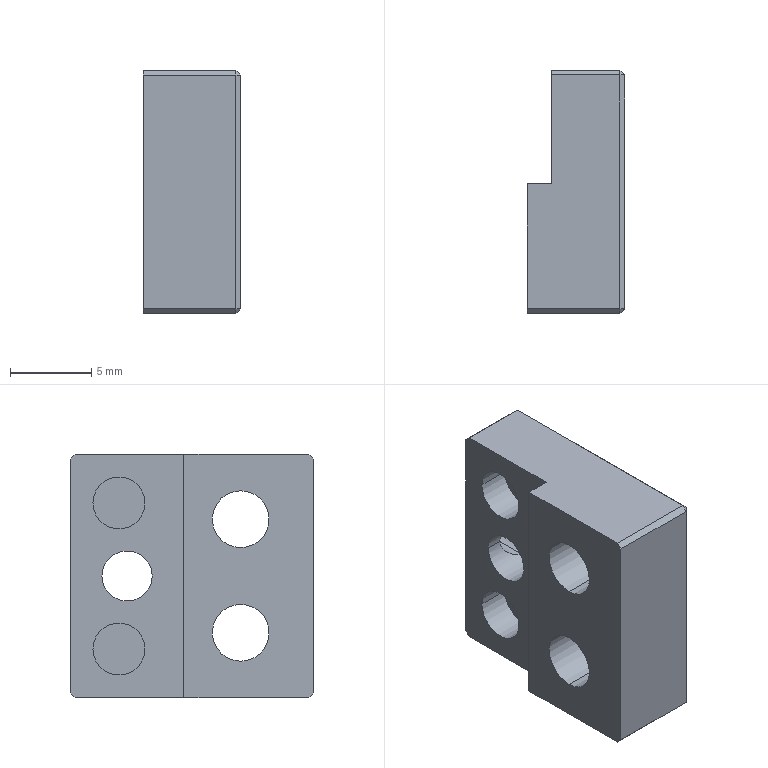Part | STEP file | Brake spring-press seat | 1 solid | 40 faces | box 6 x 15 x 15 mm | volume 832.507 mm3 | plane 24 | cylinder 16 | commonest cylinder face diameters 3.2 x4 3.5 x4 6.5 x4 2.459 x2 3.1 x2